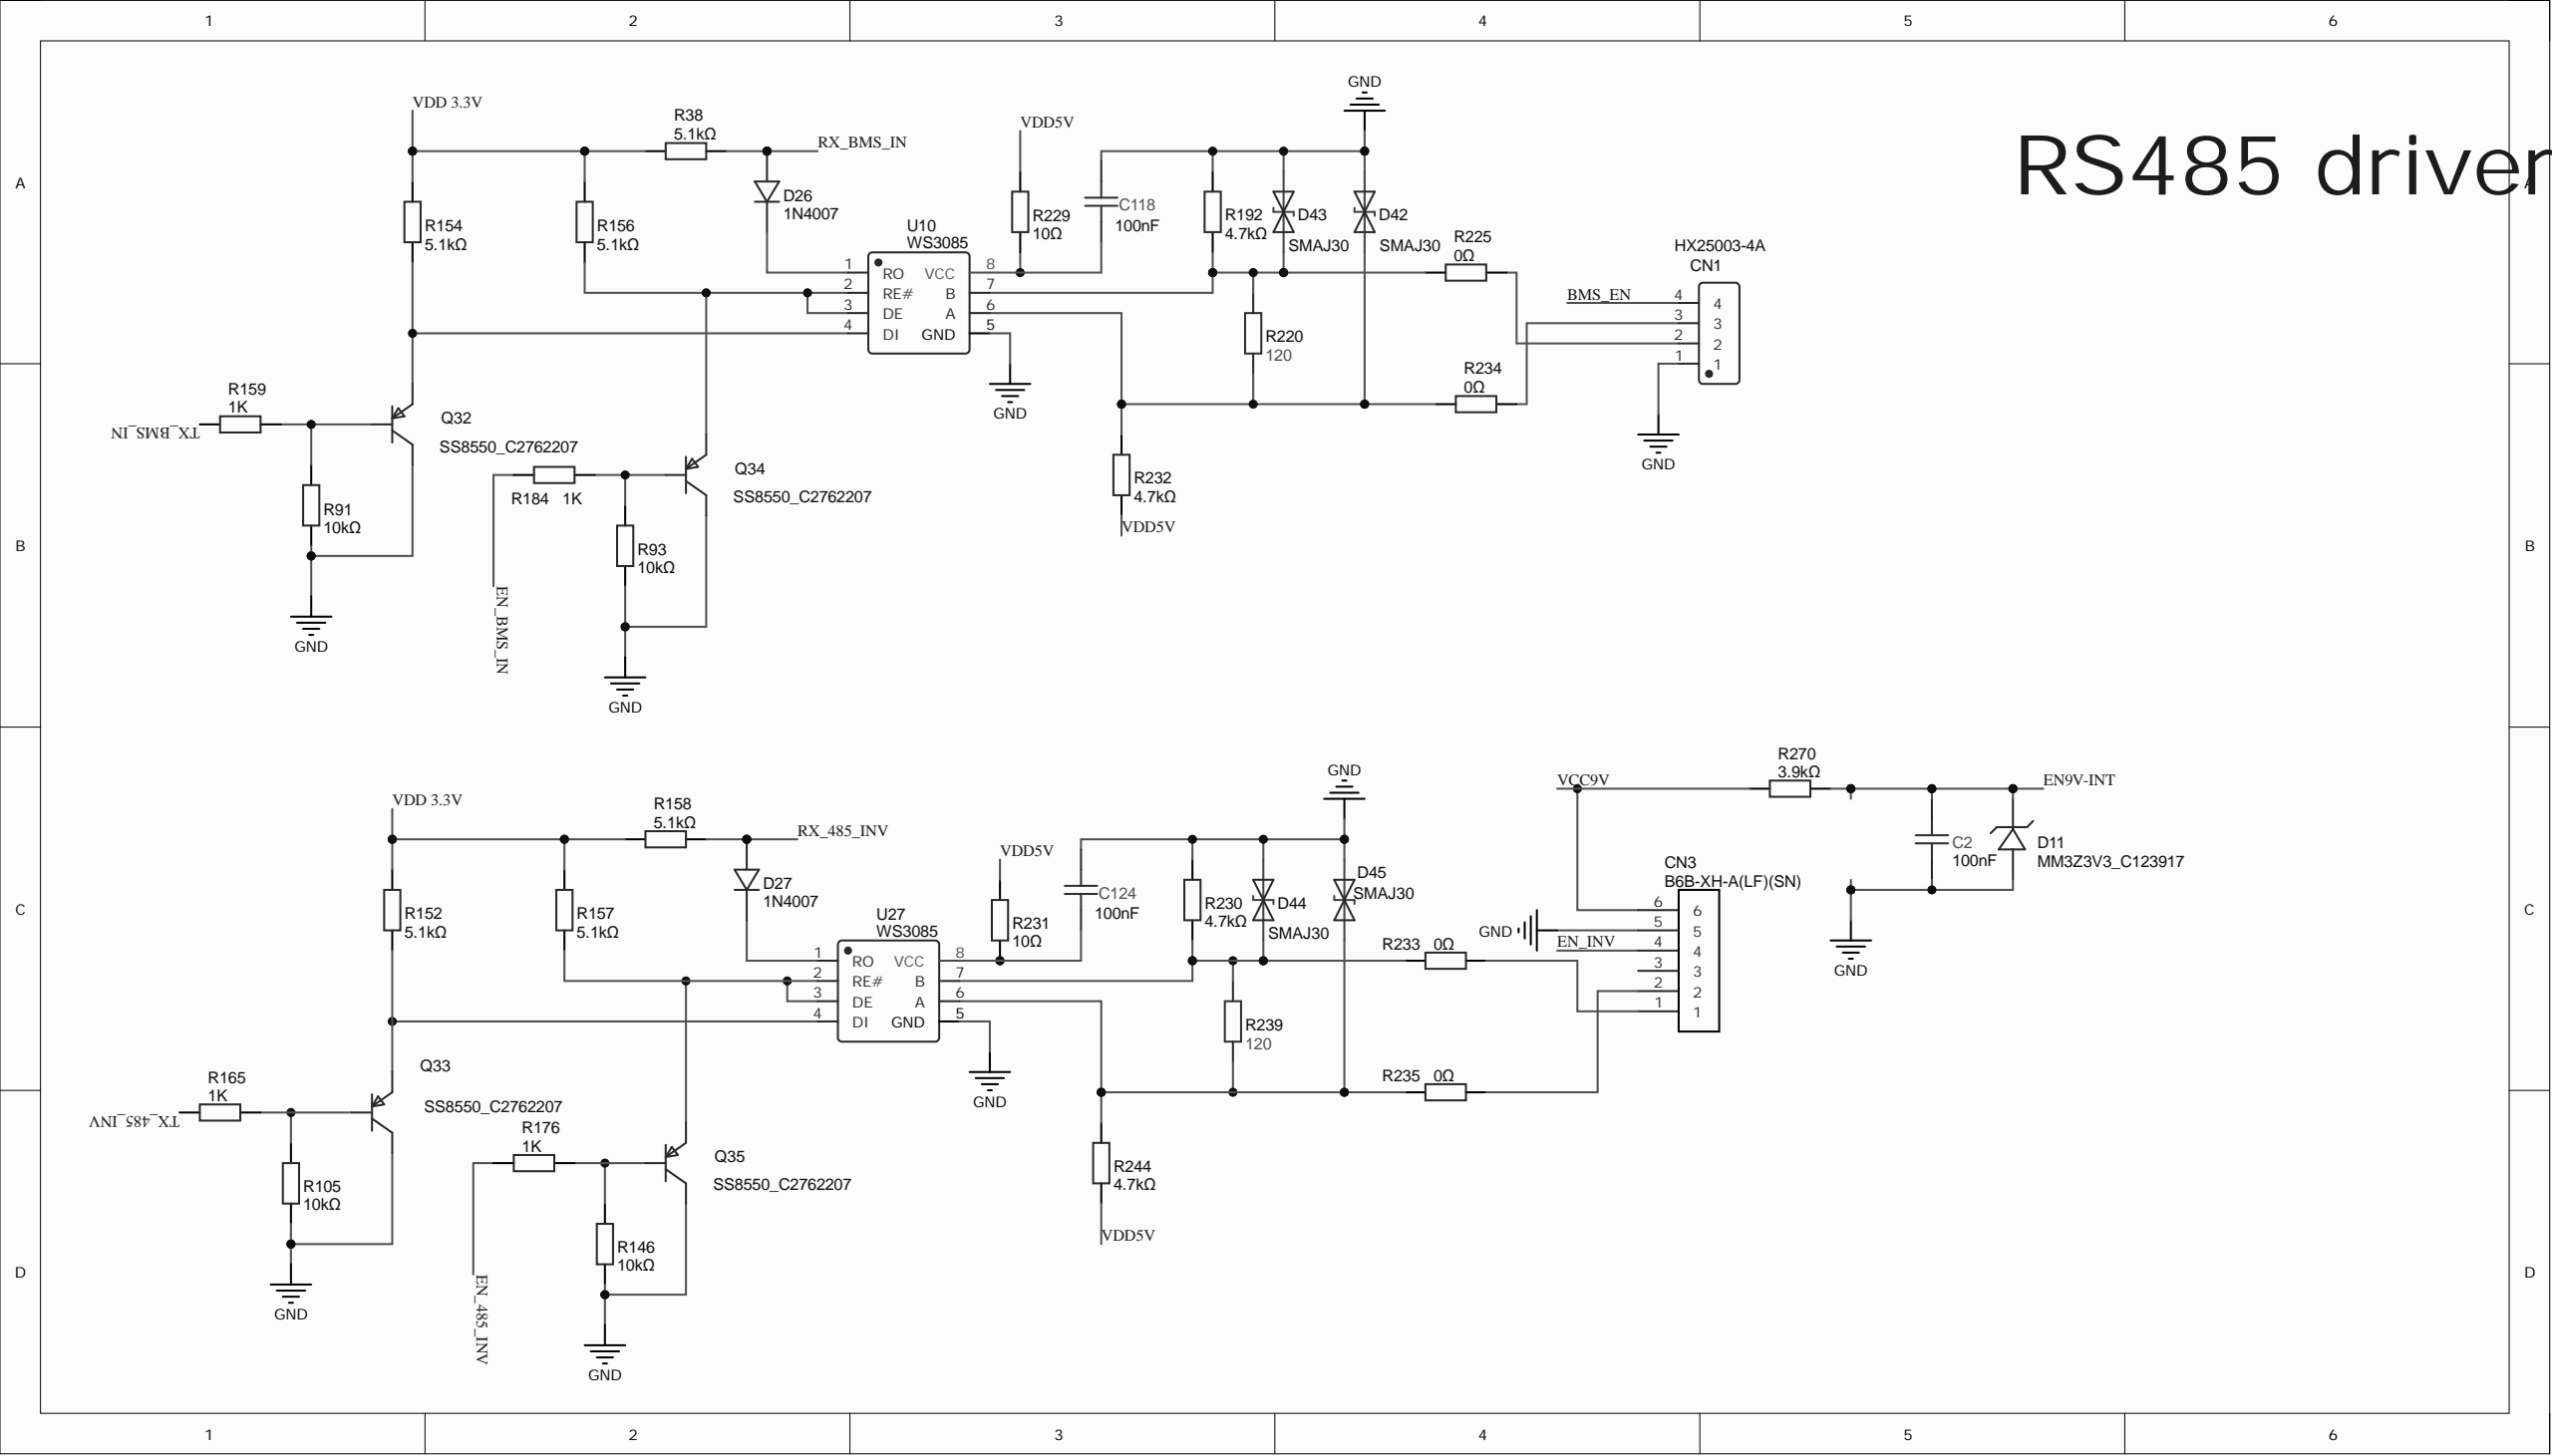Circuit board | Altium Designer | 694 parts | 423 nets | one sheet of the schematic
Parts on this sheet (reference | value | footprint):
C2 | 100nF | C0603
C124 | 100nF | C0603
CN1 | HX25003-4A | CONN-TH_4P-P2.50_HX25003-4A
CN3 | B6B-XH-A(LF)(SN) | CONN-TH_6P-P2.50_B6B-XH-A-LF-SN
D11 | MM3Z3V3_C123917 | SOD-323_L1.8-W1.3-LS2.5-RD
D26 | 1N4007 | DO-41_BD2.4-L4.7-P8.70-D0.9-RD
D27 | 1N4007 | DO-41_BD2.4-L4.7-P8.70-D0.9-RD
D42 | SMAJ30 | SMA_L4.3-W2.5-LS5.0-BI
D43 | SMAJ30 | SMA_L4.3-W2.5-LS5.0-BI
D44 | SMAJ30 | SMA_L4.3-W2.5-LS5.0-BI
D45 | SMAJ30 | SMA_L4.3-W2.5-LS5.0-BI
Q32 | SS8550_C2762207 | SOT-23-3_L2.9-W1.3-P1.90-LS2.4-BR
Q33 | SS8550_C2762207 | SOT-23-3_L2.9-W1.3-P1.90-LS2.4-BR
Q34 | SS8550_C2762207 | SOT-23-3_L2.9-W1.3-P1.90-LS2.4-BR
Q35 | SS8550_C2762207 | SOT-23-3_L2.9-W1.3-P1.90-LS2.4-BR
R38 | 5.1kΩ | R0603
R91 | 10kΩ | R0603
R93 | 10kΩ | R0603
R105 | 10kΩ | R0603
R146 | 10kΩ | R0603
R152 | 5.1kΩ | R0603
R154 | 5.1kΩ | R0603
R156 | 5.1kΩ | R0603
R157 | 5.1kΩ | R0603
R158 | 5.1kΩ | R0603
R159 | 1K | R0603
R165 | 1K | R0603
R176 | 1K | R0603
R184 | 1K | R0603
R192 | 4.7kΩ | R0603
R220 | 120 | R1206
R225 | 0Ω | R0603
R229 | 10Ω | R0603
R230 | 4.7kΩ | R0603
R231 | 10Ω | R0603
R232 | 4.7kΩ | R0603
R233 | 0Ω | R0603
R234 | 0Ω | R0603
R235 | 0Ω | R0603
R239 | 120 | R1206
R244 | 4.7kΩ | R0603
R270 | 3.9kΩ | R0603
U10 | WS3085 | SOP-8_L5.0-W4.0-P1.27-LS6.0-BL
U27 | WS3085 | SOP-8_L5.0-W4.0-P1.27-LS6.0-BL
Nets of these parts (net: part-pin ...):
VDD 3.3V: R38-1 R152-2 R154-2 R156-2 R157-2 R158-1
VDD5V: R229-2 R231-2 R232-1 R244-1
VCC9V: CN3-6 R270-1
TX_BMS_IN: R159-1
TX_485_INV: R165-1
RX_BMS_IN: D26-2 R38-2
RX_485_INV: D27-2 R158-2
NetQ35_2: Q35-2 R157-1 U27-2 U27-3
NetQ35_1: Q35-1 R146-2 R176-2
NetQ34_2: Q34-2 R156-1 U10-2 U10-3
NetQ34_1: Q34-1 R93-2 R184-2
NetQ33_2: Q33-2 R152-1 U27-4
NetQ33_1: Q33-1 R105-2 R165-2
NetQ32_2: Q32-2 R154-1 U10-4
NetQ32_1: Q32-1 R91-2 R159-2
NetD45_1: D45-1 R235-1 R239-2 R244-2 U27-6
NetD44_1: D44-1 R230-1 R233-1 R239-1 U27-7
NetD43_1: D43-1 R192-1 R220-2 R225-1 U10-7
NetD42_1: D42-1 R220-1 R232-2 R234-1 U10-6
NetD27_1: D27-1 U27-1
NetD26_1: D26-1 U10-1
NetCN3_2: CN3-2 R235-2
NetCN3_1: CN3-1 R233-2
NetCN1_3: CN1-3 R234-2
NetCN1_2: CN1-2 R225-2
NetC124_1: C124-1 R231-1 U27-8
NetC118_1: R229-1 U10-8
GND: C2-1 C124-2 CN1-1 CN3-5 D11-2 D42-2 D43-2 D44-2 D45-2 Q32-3 Q33-3 Q34-3 Q35-3 R91-1 R93-1 R105-1 R146-1 R192-2 R230-2 U10-5 U27-5
EN_INV: CN3-4
EN_BMS_IN: R184-1
EN_485_INV: R176-1
EN9V-INT: C2-2 D11-1 R270-2
BMS_EN: CN1-4